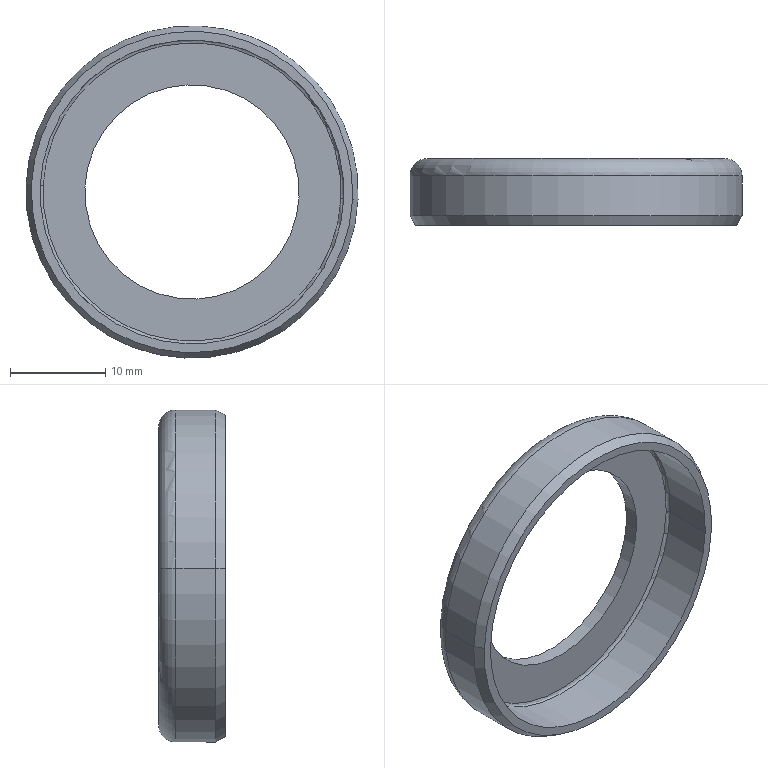Part | SolidWorks | features BaseBody 1 | 1 solid | 15 faces | box 34.9 x 7 x 34.9 mm | volume 1600 mm3 | cylinder 6 | torus 4 | plane 3 | cone 2 | commonest cylinder face diameters 22.5 x2 31.9 x2 34.9 x2
STEP:
#1=CARTESIAN_POINT('',(212.645,91.,0.7786));
#2=VERTEX_POINT('',#1);
#3=CARTESIAN_POINT('',(246.355,91.,-0.7786));
#4=VERTEX_POINT('',#3);
#5=CARTESIAN_POINT('',(229.5,91.,0.));
#6=DIRECTION('',(0.,-1.,0.));
#7=DIRECTION('',(-0.9989,0.,0.04615));
#8=AXIS2_PLACEMENT_3D('',#5,#6,#7);
#9=CIRCLE('',#8,16.873);
#10=EDGE_CURVE('',#2,#4,#9,.T.);
#11=ORIENTED_EDGE('',*,*,#10,.F.);
#12=CARTESIAN_POINT('',(212.069,92.,0.8053));
#13=VERTEX_POINT('',#12);
#14=CARTESIAN_POINT('',(212.645,91.,0.7786));
#15=DIRECTION('',(-0.4995,0.866,0.02307));
#16=VECTOR('',#15,1000.);
#17=LINE('',#14,#16);
#18=EDGE_CURVE('',#2,#13,#17,.T.);
#19=ORIENTED_EDGE('',*,*,#18,.T.);
#20=CARTESIAN_POINT('',(246.931,92.,-0.8053));
#21=VERTEX_POINT('',#20);
#22=CARTESIAN_POINT('',(229.5,92.,0.));
#23=DIRECTION('',(0.,1.,0.));
#24=DIRECTION('',(-0.9989,0.,0.04615));
#25=AXIS2_PLACEMENT_3D('',#22,#23,#24);
#26=CIRCLE('',#25,17.45);
#27=EDGE_CURVE('',#21,#13,#26,.T.);
#28=ORIENTED_EDGE('',*,*,#27,.F.);
#29=CARTESIAN_POINT('',(246.355,91.,-0.7786));
#30=DIRECTION('',(0.4995,0.866,-0.02307));
#31=VECTOR('',#30,1000.);
#32=LINE('',#29,#31);
#33=EDGE_CURVE('',#4,#21,#32,.T.);
#34=ORIENTED_EDGE('',*,*,#33,.F.);
#35=EDGE_LOOP('',(#11,#19,#28,#34));
#36=FACE_OUTER_BOUND('',#35,.T.);
#37=CARTESIAN_POINT('',(229.5,91.,0.));
#38=DIRECTION('',(0.,1.,0.));
#39=DIRECTION('',(0.9989,0.,-0.04615));
#40=AXIS2_PLACEMENT_3D('',#37,#38,#39);
#41=CONICAL_SURFACE('',#40,16.873,0.5236);
#42=ADVANCED_FACE('',(#36),#41,.T.);
#43=CARTESIAN_POINT('',(245.133,96.5,-0.7222));
#44=VERTEX_POINT('',#43);
#45=CARTESIAN_POINT('',(213.867,96.5,0.7222));
#46=VERTEX_POINT('',#45);
#47=CARTESIAN_POINT('',(229.5,96.5,0.));
#48=DIRECTION('',(0.,-1.,0.));
#49=DIRECTION('',(-0.9989,0.,0.04615));
#50=AXIS2_PLACEMENT_3D('',#47,#48,#49);
#51=CIRCLE('',#50,15.65);
#52=EDGE_CURVE('',#44,#46,#51,.T.);
#53=ORIENTED_EDGE('',*,*,#52,.F.);
#54=CARTESIAN_POINT('',(245.433,96.2,-0.7361));
#55=VERTEX_POINT('',#54);
#56=CARTESIAN_POINT('',(245.133,96.2,-0.7222));
#57=DIRECTION('',(-0.04615,0.,-0.9989));
#58=DIRECTION('',(-0.9989,0.,0.04615));
#59=AXIS2_PLACEMENT_3D('',#56,#57,#58);
#60=CIRCLE('',#59,0.3);
#61=EDGE_CURVE('',#44,#55,#60,.T.);
#62=ORIENTED_EDGE('',*,*,#61,.T.);
#63=CARTESIAN_POINT('',(213.567,96.2,0.7361));
#64=VERTEX_POINT('',#63);
#65=CARTESIAN_POINT('',(229.5,96.2,0.));
#66=DIRECTION('',(0.,1.,0.));
#67=DIRECTION('',(-0.9989,0.,0.04615));
#68=AXIS2_PLACEMENT_3D('',#65,#66,#67);
#69=CIRCLE('',#68,15.95);
#70=EDGE_CURVE('',#64,#55,#69,.T.);
#71=ORIENTED_EDGE('',*,*,#70,.F.);
#72=CARTESIAN_POINT('',(213.867,96.2,0.7222));
#73=DIRECTION('',(0.04615,0.,0.9989));
#74=DIRECTION('',(0.9989,0.,-0.04615));
#75=AXIS2_PLACEMENT_3D('',#72,#73,#74);
#76=CIRCLE('',#75,0.3);
#77=EDGE_CURVE('',#46,#64,#76,.T.);
#78=ORIENTED_EDGE('',*,*,#77,.F.);
#79=EDGE_LOOP('',(#53,#62,#71,#78));
#80=FACE_OUTER_BOUND('',#79,.T.);
#81=CARTESIAN_POINT('',(229.5,96.2,0.));
#82=DIRECTION('',(0.,-1.,0.));
#83=DIRECTION('',(-0.9989,0.,0.04615));
#84=AXIS2_PLACEMENT_3D('',#81,#82,#83);
#85=TOROIDAL_SURFACE('',#84,15.65,0.3);
#86=ADVANCED_FACE('',(#80),#85,.F.);
#87=CARTESIAN_POINT('',(240.738,96.5,-0.5192));
#88=VERTEX_POINT('',#87);
#89=CARTESIAN_POINT('',(218.262,96.5,0.5192));
#90=VERTEX_POINT('',#89);
#91=CARTESIAN_POINT('',(229.5,96.5,0.));
#92=DIRECTION('',(0.,-1.,0.));
#93=DIRECTION('',(-0.9989,0.,0.04615));
#94=AXIS2_PLACEMENT_3D('',#91,#92,#93);
#95=CIRCLE('',#94,11.25);
#96=EDGE_CURVE('',#88,#90,#95,.T.);
#97=ORIENTED_EDGE('',*,*,#96,.T.);
#98=CARTESIAN_POINT('',(218.262,98.,0.5192));
#99=VERTEX_POINT('',#98);
#100=CARTESIAN_POINT('',(218.262,91.,0.5192));
#101=DIRECTION('',(0.,1.,0.));
#102=VECTOR('',#101,1000.);
#103=LINE('',#100,#102);
#104=EDGE_CURVE('',#90,#99,#103,.T.);
#105=ORIENTED_EDGE('',*,*,#104,.T.);
#106=CARTESIAN_POINT('',(240.738,98.,-0.5192));
#107=VERTEX_POINT('',#106);
#108=CARTESIAN_POINT('',(229.5,98.,0.));
#109=DIRECTION('',(0.,1.,0.));
#110=DIRECTION('',(0.9989,0.,-0.04615));
#111=AXIS2_PLACEMENT_3D('',#108,#109,#110);
#112=CIRCLE('',#111,11.25);
#113=EDGE_CURVE('',#99,#107,#112,.T.);
#114=ORIENTED_EDGE('',*,*,#113,.T.);
#115=CARTESIAN_POINT('',(240.738,91.,-0.5192));
#116=DIRECTION('',(0.,1.,0.));
#117=VECTOR('',#116,1000.);
#118=LINE('',#115,#117);
#119=EDGE_CURVE('',#88,#107,#118,.T.);
#120=ORIENTED_EDGE('',*,*,#119,.F.);
#121=EDGE_LOOP('',(#97,#105,#114,#120));
#122=FACE_OUTER_BOUND('',#121,.T.);
#123=CARTESIAN_POINT('',(229.5,91.,0.));
#124=DIRECTION('',(0.,1.,0.));
#125=DIRECTION('',(0.9989,0.,-0.04615));
#126=AXIS2_PLACEMENT_3D('',#123,#124,#125);
#127=CYLINDRICAL_SURFACE('',#126,11.25);
#128=ADVANCED_FACE('',(#122),#127,.F.);
#129=CARTESIAN_POINT('',(245.133,98.,-0.7222));
#130=VERTEX_POINT('',#129);
#131=CARTESIAN_POINT('',(213.867,98.,0.7222));
#132=VERTEX_POINT('',#131);
#133=CARTESIAN_POINT('',(229.5,98.,0.));
#134=DIRECTION('',(0.,1.,0.));
#135=DIRECTION('',(-0.9989,0.,0.04615));
#136=AXIS2_PLACEMENT_3D('',#133,#134,#135);
#137=CIRCLE('',#136,15.65);
#138=EDGE_CURVE('',#130,#132,#137,.T.);
#139=ORIENTED_EDGE('',*,*,#138,.F.);
#140=CARTESIAN_POINT('',(246.931,96.2,-0.8053));
#141=VERTEX_POINT('',#140);
#142=CARTESIAN_POINT('',(245.133,96.2,-0.7222));
#143=DIRECTION('',(-0.04615,0.,-0.9989));
#144=DIRECTION('',(-0.9989,0.,0.04615));
#145=AXIS2_PLACEMENT_3D('',#142,#143,#144);
#146=CIRCLE('',#145,1.8);
#147=EDGE_CURVE('',#130,#141,#146,.T.);
#148=ORIENTED_EDGE('',*,*,#147,.T.);
#149=CARTESIAN_POINT('',(212.069,96.2,0.8053));
#150=VERTEX_POINT('',#149);
#151=CARTESIAN_POINT('',(229.5,96.2,0.));
#152=DIRECTION('',(0.,-1.,0.));
#153=DIRECTION('',(-0.9989,0.,0.04615));
#154=AXIS2_PLACEMENT_3D('',#151,#152,#153);
#155=CIRCLE('',#154,17.45);
#156=EDGE_CURVE('',#150,#141,#155,.T.);
#157=ORIENTED_EDGE('',*,*,#156,.F.);
#158=CARTESIAN_POINT('',(213.867,96.2,0.7222));
#159=DIRECTION('',(0.04615,0.,0.9989));
#160=DIRECTION('',(0.9989,0.,-0.04615));
#161=AXIS2_PLACEMENT_3D('',#158,#159,#160);
#162=CIRCLE('',#161,1.8);
#163=EDGE_CURVE('',#132,#150,#162,.T.);
#164=ORIENTED_EDGE('',*,*,#163,.F.);
#165=EDGE_LOOP('',(#139,#148,#157,#164));
#166=FACE_OUTER_BOUND('',#165,.T.);
#167=CARTESIAN_POINT('',(229.5,96.2,0.));
#168=DIRECTION('',(0.,-1.,0.));
#169=DIRECTION('',(-0.9989,0.,0.04615));
#170=AXIS2_PLACEMENT_3D('',#167,#168,#169);
#171=TOROIDAL_SURFACE('',#170,15.65,1.8);
#172=ADVANCED_FACE('',(#166),#171,.T.);
#173=ORIENTED_EDGE('',*,*,#70,.T.);
#174=CARTESIAN_POINT('',(245.433,91.,-0.7361));
#175=VERTEX_POINT('',#174);
#176=CARTESIAN_POINT('',(245.433,143.113,-0.7361));
#177=DIRECTION('',(0.,-1.,0.));
#178=VECTOR('',#177,1000.);
#179=LINE('',#176,#178);
#180=EDGE_CURVE('',#55,#175,#179,.T.);
#181=ORIENTED_EDGE('',*,*,#180,.T.);
#182=CARTESIAN_POINT('',(213.567,91.,0.7361));
#183=VERTEX_POINT('',#182);
#184=CARTESIAN_POINT('',(229.5,91.,0.));
#185=DIRECTION('',(0.,-1.,0.));
#186=DIRECTION('',(-0.9989,0.,0.04615));
#187=AXIS2_PLACEMENT_3D('',#184,#185,#186);
#188=CIRCLE('',#187,15.95);
#189=EDGE_CURVE('',#175,#183,#188,.T.);
#190=ORIENTED_EDGE('',*,*,#189,.T.);
#191=CARTESIAN_POINT('',(213.567,143.113,0.7361));
#192=DIRECTION('',(0.,-1.,0.));
#193=VECTOR('',#192,1000.);
#194=LINE('',#191,#193);
#195=EDGE_CURVE('',#64,#183,#194,.T.);
#196=ORIENTED_EDGE('',*,*,#195,.F.);
#197=EDGE_LOOP('',(#173,#181,#190,#196));
#198=FACE_OUTER_BOUND('',#197,.T.);
#199=CARTESIAN_POINT('',(229.5,143.113,0.));
#200=DIRECTION('',(0.,-1.,0.));
#201=DIRECTION('',(-0.9989,0.,0.04615));
#202=AXIS2_PLACEMENT_3D('',#199,#200,#201);
#203=CYLINDRICAL_SURFACE('',#202,15.95);
#204=ADVANCED_FACE('',(#198),#203,.F.);
#205=ORIENTED_EDGE('',*,*,#27,.T.);
#206=CARTESIAN_POINT('',(212.069,91.,0.8053));
#207=DIRECTION('',(0.,1.,0.));
#208=VECTOR('',#207,1000.);
#209=LINE('',#206,#208);
#210=EDGE_CURVE('',#13,#150,#209,.T.);
#211=ORIENTED_EDGE('',*,*,#210,.T.);
#212=ORIENTED_EDGE('',*,*,#156,.T.);
#213=CARTESIAN_POINT('',(246.931,91.,-0.8053));
#214=DIRECTION('',(0.,1.,0.));
#215=VECTOR('',#214,1000.);
#216=LINE('',#213,#215);
#217=EDGE_CURVE('',#21,#141,#216,.T.);
#218=ORIENTED_EDGE('',*,*,#217,.F.);
#219=EDGE_LOOP('',(#205,#211,#212,#218));
#220=FACE_OUTER_BOUND('',#219,.T.);
#221=CARTESIAN_POINT('',(229.5,91.,0.));
#222=DIRECTION('',(0.,1.,0.));
#223=DIRECTION('',(0.9989,0.,-0.04615));
#224=AXIS2_PLACEMENT_3D('',#221,#222,#223);
#225=CYLINDRICAL_SURFACE('',#224,17.45);
#226=ADVANCED_FACE('',(#220),#225,.T.);
#227=ORIENTED_EDGE('',*,*,#210,.F.);
#228=CARTESIAN_POINT('',(229.5,92.,0.));
#229=DIRECTION('',(0.,1.,0.));
#230=DIRECTION('',(-0.9989,0.,0.04615));
#231=AXIS2_PLACEMENT_3D('',#228,#229,#230);
#232=CIRCLE('',#231,17.45);
#233=EDGE_CURVE('',#13,#21,#232,.T.);
#234=ORIENTED_EDGE('',*,*,#233,.T.);
#235=ORIENTED_EDGE('',*,*,#217,.T.);
#236=CARTESIAN_POINT('',(229.5,96.2,0.));
#237=DIRECTION('',(0.,-1.,0.));
#238=DIRECTION('',(-0.9989,0.,0.04615));
#239=AXIS2_PLACEMENT_3D('',#236,#237,#238);
#240=CIRCLE('',#239,17.45);
#241=EDGE_CURVE('',#141,#150,#240,.T.);
#242=ORIENTED_EDGE('',*,*,#241,.T.);
#243=EDGE_LOOP('',(#227,#234,#235,#242));
#244=FACE_OUTER_BOUND('',#243,.T.);
#245=CARTESIAN_POINT('',(229.5,91.,0.));
#246=DIRECTION('',(0.,1.,0.));
#247=DIRECTION('',(0.9989,0.,-0.04615));
#248=AXIS2_PLACEMENT_3D('',#245,#246,#247);
#249=CYLINDRICAL_SURFACE('',#248,17.45);
#250=ADVANCED_FACE('',(#244),#249,.T.);
#251=CARTESIAN_POINT('',(229.5,91.,0.));
#252=DIRECTION('',(0.,-1.,0.));
#253=DIRECTION('',(-0.9989,0.,0.04615));
#254=AXIS2_PLACEMENT_3D('',#251,#252,#253);
#255=CIRCLE('',#254,16.873);
#256=EDGE_CURVE('',#4,#2,#255,.T.);
#257=ORIENTED_EDGE('',*,*,#256,.T.);
#258=ORIENTED_EDGE('',*,*,#10,.T.);
#259=EDGE_LOOP('',(#257,#258));
#260=FACE_OUTER_BOUND('',#259,.T.);
#261=CARTESIAN_POINT('',(229.5,91.,0.));
#262=DIRECTION('',(0.,-1.,0.));
#263=DIRECTION('',(-0.9989,0.,0.04615));
#264=AXIS2_PLACEMENT_3D('',#261,#262,#263);
#265=CIRCLE('',#264,15.95);
#266=EDGE_CURVE('',#183,#175,#265,.T.);
#267=ORIENTED_EDGE('',*,*,#266,.F.);
#268=ORIENTED_EDGE('',*,*,#189,.F.);
#269=EDGE_LOOP('',(#267,#268));
#270=FACE_BOUND('',#269,.T.);
#271=CARTESIAN_POINT('',(229.5,91.,0.));
#272=DIRECTION('',(0.,-1.,0.));
#273=DIRECTION('',(-0.9989,0.,0.04615));
#274=AXIS2_PLACEMENT_3D('',#271,#272,#273);
#275=PLANE('',#274);
#276=ADVANCED_FACE('',(#260,#270),#275,.T.);
#277=CARTESIAN_POINT('',(229.5,98.,0.));
#278=DIRECTION('',(0.,1.,0.));
#279=DIRECTION('',(0.9989,0.,-0.04615));
#280=AXIS2_PLACEMENT_3D('',#277,#278,#279);
#281=CIRCLE('',#280,11.25);
#282=EDGE_CURVE('',#107,#99,#281,.T.);
#283=ORIENTED_EDGE('',*,*,#282,.F.);
#284=ORIENTED_EDGE('',*,*,#113,.F.);
#285=EDGE_LOOP('',(#283,#284));
#286=FACE_BOUND('',#285,.T.);
#287=CARTESIAN_POINT('',(229.5,98.,0.));
#288=DIRECTION('',(0.,1.,0.));
#289=DIRECTION('',(-0.9989,0.,0.04615));
#290=AXIS2_PLACEMENT_3D('',#287,#288,#289);
#291=CIRCLE('',#290,15.65);
#292=EDGE_CURVE('',#132,#130,#291,.T.);
#293=ORIENTED_EDGE('',*,*,#292,.T.);
#294=ORIENTED_EDGE('',*,*,#138,.T.);
#295=EDGE_LOOP('',(#293,#294));
#296=FACE_OUTER_BOUND('',#295,.T.);
#297=CARTESIAN_POINT('',(229.5,98.,0.));
#298=DIRECTION('',(0.,-1.,0.));
#299=DIRECTION('',(-0.9989,0.,0.04615));
#300=AXIS2_PLACEMENT_3D('',#297,#298,#299);
#301=PLANE('',#300);
#302=ADVANCED_FACE('',(#286,#296),#301,.F.);
#303=ORIENTED_EDGE('',*,*,#180,.F.);
#304=CARTESIAN_POINT('',(229.5,96.2,0.));
#305=DIRECTION('',(0.,1.,0.));
#306=DIRECTION('',(-0.9989,0.,0.04615));
#307=AXIS2_PLACEMENT_3D('',#304,#305,#306);
#308=CIRCLE('',#307,15.95);
#309=EDGE_CURVE('',#55,#64,#308,.T.);
#310=ORIENTED_EDGE('',*,*,#309,.T.);
#311=ORIENTED_EDGE('',*,*,#195,.T.);
#312=ORIENTED_EDGE('',*,*,#266,.T.);
#313=EDGE_LOOP('',(#303,#310,#311,#312));
#314=FACE_OUTER_BOUND('',#313,.T.);
#315=CARTESIAN_POINT('',(229.5,143.113,0.));
#316=DIRECTION('',(0.,-1.,0.));
#317=DIRECTION('',(-0.9989,0.,0.04615));
#318=AXIS2_PLACEMENT_3D('',#315,#316,#317);
#319=CYLINDRICAL_SURFACE('',#318,15.95);
#320=ADVANCED_FACE('',(#314),#319,.F.);
#321=CARTESIAN_POINT('',(229.5,96.5,0.));
#322=DIRECTION('',(0.,-1.,0.));
#323=DIRECTION('',(-0.9989,0.,0.04615));
#324=AXIS2_PLACEMENT_3D('',#321,#322,#323);
#325=CIRCLE('',#324,15.65);
#326=EDGE_CURVE('',#46,#44,#325,.T.);
#327=ORIENTED_EDGE('',*,*,#326,.T.);
#328=ORIENTED_EDGE('',*,*,#52,.T.);
#329=EDGE_LOOP('',(#327,#328));
#330=FACE_OUTER_BOUND('',#329,.T.);
#331=ORIENTED_EDGE('',*,*,#96,.F.);
#332=CARTESIAN_POINT('',(229.5,96.5,0.));
#333=DIRECTION('',(0.,-1.,0.));
#334=DIRECTION('',(-0.9989,0.,0.04615));
#335=AXIS2_PLACEMENT_3D('',#332,#333,#334);
#336=CIRCLE('',#335,11.25);
#337=EDGE_CURVE('',#90,#88,#336,.T.);
#338=ORIENTED_EDGE('',*,*,#337,.F.);
#339=EDGE_LOOP('',(#331,#338));
#340=FACE_BOUND('',#339,.T.);
#341=CARTESIAN_POINT('',(229.5,96.5,0.));
#342=DIRECTION('',(0.,-1.,0.));
#343=DIRECTION('',(-0.9989,0.,0.04615));
#344=AXIS2_PLACEMENT_3D('',#341,#342,#343);
#345=PLANE('',#344);
#346=ADVANCED_FACE('',(#330,#340),#345,.T.);
#347=ORIENTED_EDGE('',*,*,#147,.F.);
#348=ORIENTED_EDGE('',*,*,#292,.F.);
#349=ORIENTED_EDGE('',*,*,#163,.T.);
#350=ORIENTED_EDGE('',*,*,#241,.F.);
#351=EDGE_LOOP('',(#347,#348,#349,#350));
#352=FACE_OUTER_BOUND('',#351,.T.);
#353=CARTESIAN_POINT('',(229.5,96.2,0.));
#354=DIRECTION('',(0.,-1.,0.));
#355=DIRECTION('',(-0.9989,0.,0.04615));
#356=AXIS2_PLACEMENT_3D('',#353,#354,#355);
#357=TOROIDAL_SURFACE('',#356,15.65,1.8);
#358=ADVANCED_FACE('',(#352),#357,.T.);
#359=ORIENTED_EDGE('',*,*,#104,.F.);
#360=ORIENTED_EDGE('',*,*,#337,.T.);
#361=ORIENTED_EDGE('',*,*,#119,.T.);
#362=ORIENTED_EDGE('',*,*,#282,.T.);
#363=EDGE_LOOP('',(#359,#360,#361,#362));
#364=FACE_OUTER_BOUND('',#363,.T.);
#365=CARTESIAN_POINT('',(229.5,91.,0.));
#366=DIRECTION('',(0.,1.,0.));
#367=DIRECTION('',(0.9989,0.,-0.04615));
#368=AXIS2_PLACEMENT_3D('',#365,#366,#367);
#369=CYLINDRICAL_SURFACE('',#368,11.25);
#370=ADVANCED_FACE('',(#364),#369,.F.);
#371=ORIENTED_EDGE('',*,*,#61,.F.);
#372=ORIENTED_EDGE('',*,*,#326,.F.);
#373=ORIENTED_EDGE('',*,*,#77,.T.);
#374=ORIENTED_EDGE('',*,*,#309,.F.);
#375=EDGE_LOOP('',(#371,#372,#373,#374));
#376=FACE_OUTER_BOUND('',#375,.T.);
#377=CARTESIAN_POINT('',(229.5,96.2,0.));
#378=DIRECTION('',(0.,-1.,0.));
#379=DIRECTION('',(-0.9989,0.,0.04615));
#380=AXIS2_PLACEMENT_3D('',#377,#378,#379);
#381=TOROIDAL_SURFACE('',#380,15.65,0.3);
#382=ADVANCED_FACE('',(#376),#381,.F.);
#383=ORIENTED_EDGE('',*,*,#18,.F.);
#384=ORIENTED_EDGE('',*,*,#256,.F.);
#385=ORIENTED_EDGE('',*,*,#33,.T.);
#386=ORIENTED_EDGE('',*,*,#233,.F.);
#387=EDGE_LOOP('',(#383,#384,#385,#386));
#388=FACE_OUTER_BOUND('',#387,.T.);
#389=CARTESIAN_POINT('',(229.5,91.,0.));
#390=DIRECTION('',(0.,1.,0.));
#391=DIRECTION('',(0.9989,0.,-0.04615));
#392=AXIS2_PLACEMENT_3D('',#389,#390,#391);
#393=CONICAL_SURFACE('',#392,16.873,0.5236);
#394=ADVANCED_FACE('',(#388),#393,.T.);
#395=CLOSED_SHELL('',(#42,#86,#128,#172,#204,#226,#250,#276,#302,#320,#346,#358,#370,#382,#394));
#396=MANIFOLD_SOLID_BREP('',#395);
#397=CARTESIAN_POINT('',(0.,0.,0.));
#398=DIRECTION('',(0.,0.,1.));
#399=DIRECTION('',(1.,0.,0.));
#400=AXIS2_PLACEMENT_3D('',#397,#398,#399);
#401=(LENGTH_UNIT()NAMED_UNIT(*)SI_UNIT(.MILLI.,.METRE.));
#402=UNCERTAINTY_MEASURE_WITH_UNIT(LENGTH_MEASURE(0.00001),#401,'','');
#403=(NAMED_UNIT(*)PLANE_ANGLE_UNIT()SI_UNIT($,.RADIAN.));
#404=(NAMED_UNIT(*)SI_UNIT($,.STERADIAN.)SOLID_ANGLE_UNIT());
#405=(GEOMETRIC_REPRESENTATION_CONTEXT(3)GLOBAL_UNCERTAINTY_ASSIGNED_CONTEXT((#402))GLOBAL_UNIT_ASSIGNED_CONTEXT((#401,#403,#404))REPRESENTATION_CONTEXT('',''));
#406=ADVANCED_BREP_SHAPE_REPRESENTATION('',(#396,#400),#405);